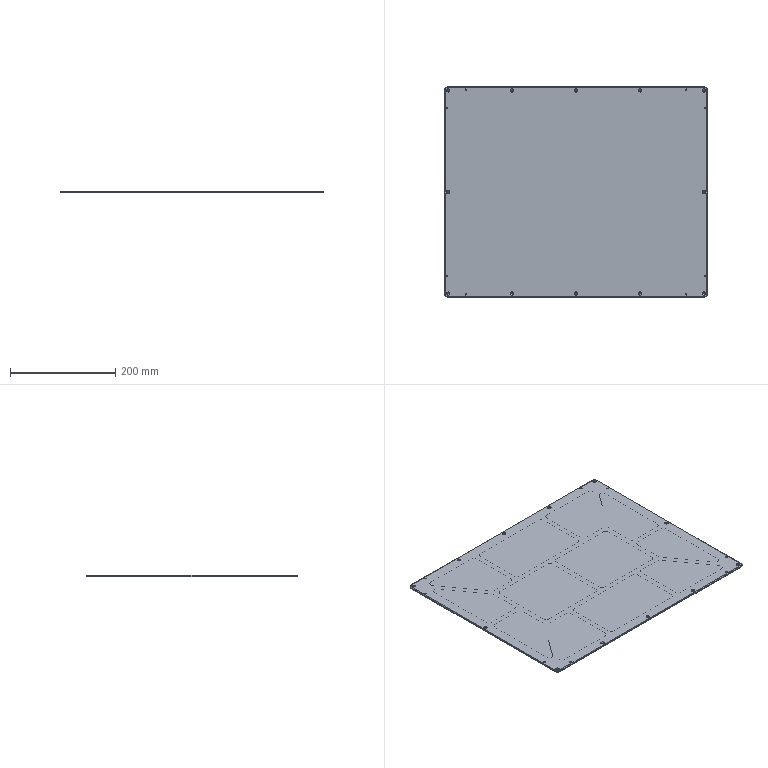CAM job | Mastercam | 3-axis milling, 5-axis milling, drilling | part box 500 x 400 x 3 mm | stock box 505 x 405 x 3 mm
Tools:
tool_number,name,type,diameter_mm,corner_radius_mm,flutes,flute_length_mm,overall_length_mm,shoulder_length_mm,holder_diameter_mm,length_offset,diameter_offset,default_rpm,default_feed_mm_min,default_plunge_mm_min,coolant
5,4 Chamfer Mill,chamfer mill,4,0,4,25,75,30,50,5,5,6250,750,600,COOL_OFF
8,8 Flat End Mill,end mill,8,0,4,25,75,25,50,8,8,1250,150,600,COOL_OFF
9,10 Flat End Mill,end mill,10,0,4,25,75,25,50,9,9,10000,5000,600,COOL_OFF
10,10 Flat End Mill,end mill,10,0,4,25,75,25,50,10,10,7000,1000,600,COOL_OFF
18,8 Bull Nose Mill,bull end mill,8,1,4,25,100,25,50,18,18,1500,180,600,COOL_OFF
Operations:
seq,operation,operation_type,tool_number,tool_name,tool_diameter_mm,spindle_rpm,feed_mm_min,plunge_mm_min,retract_mm_min,cycle_time_s,wcs,posted,nc_file
1,Contour (Ramp) - [WCS: Plane] - [Tplane: Plane],Contour,9,10 Flat End Mill,10,10000,5000,600,1200,152.541,Plane,yes,.nc
2,Contour (2D) - [WCS: Plane] - [Tplane: Plane],Contour,10,10 Flat End Mill,10,7000,1000,600,1200,110.595,Plane,yes,.nc
3,Unified Morph - [WCS: Plane] - [Tplane: Plane],461,18,8 Bull Nose Mill,8,7000,4000,600,1200,436.088,Plane,yes,.nc
4,Drill/Counterbore - [WCS: Plane] - [Tplane: Plane],Drill,5,4 Chamfer Mill,4,6000,200,600,1200,19.771,Plane,yes,.nc
5,2D High Speed (2D Area Mill) - [WCS: Plane-1] - [Tplane: Plane-1],HighSpeed2D,8,8 Flat End Mill,8,7000,3500,600,1200,3941.536,Plane-1,yes,.nc
6,Contour (2D) - [WCS: Plane-1] - [Tplane: Plane-1],Contour,8,8 Flat End Mill,8,7000,1000,600,1200,314.573,Plane-1,yes,.nc
7,Contour (2D chamfer) - [WCS: Plane-1] - [Tplane: Plane-1],Contour,5,4 Chamfer Mill,4,7000,1000,600,1200,327.241,Plane-1,yes,.nc